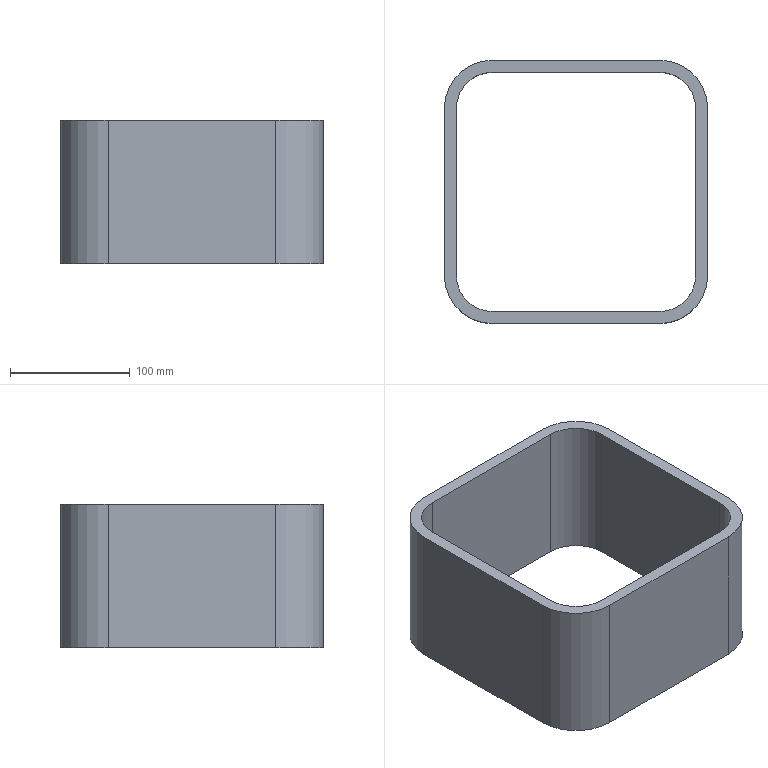Part | SolidWorks | features Extrusion 1 | 1 solid | 18 faces | box 220 x 220 x 120 mm | volume 935894 mm3 | plane 10 | cylinder 8 | commonest cylinder face diameters 60 x4 80 x4
STEP:
#1=CARTESIAN_POINT('',(-70.,110.,120.));
#2=VERTEX_POINT('',#1);
#3=CARTESIAN_POINT('',(-110.,70.,120.));
#4=VERTEX_POINT('',#3);
#5=CARTESIAN_POINT('',(-70.,70.,120.));
#6=DIRECTION('',(0.,0.,1.));
#7=DIRECTION('',(-1.,0.,0.));
#8=AXIS2_PLACEMENT_3D('',#5,#6,#7);
#9=CIRCLE('',#8,40.);
#10=EDGE_CURVE('',#2,#4,#9,.T.);
#11=ORIENTED_EDGE('',*,*,#10,.T.);
#12=CARTESIAN_POINT('',(-110.,-70.,120.));
#13=VERTEX_POINT('',#12);
#14=CARTESIAN_POINT('',(-110.,70.,120.));
#15=DIRECTION('',(0.,-1.,0.));
#16=VECTOR('',#15,1000.);
#17=LINE('',#14,#16);
#18=EDGE_CURVE('',#4,#13,#17,.T.);
#19=ORIENTED_EDGE('',*,*,#18,.T.);
#20=CARTESIAN_POINT('',(-70.,-110.,120.));
#21=VERTEX_POINT('',#20);
#22=CARTESIAN_POINT('',(-70.,-70.,120.));
#23=DIRECTION('',(0.,0.,1.));
#24=DIRECTION('',(-1.,0.,0.));
#25=AXIS2_PLACEMENT_3D('',#22,#23,#24);
#26=CIRCLE('',#25,40.);
#27=EDGE_CURVE('',#13,#21,#26,.T.);
#28=ORIENTED_EDGE('',*,*,#27,.T.);
#29=CARTESIAN_POINT('',(70.,-110.,120.));
#30=VERTEX_POINT('',#29);
#31=CARTESIAN_POINT('',(-70.,-110.,120.));
#32=DIRECTION('',(1.,0.,0.));
#33=VECTOR('',#32,1000.);
#34=LINE('',#31,#33);
#35=EDGE_CURVE('',#21,#30,#34,.T.);
#36=ORIENTED_EDGE('',*,*,#35,.T.);
#37=CARTESIAN_POINT('',(110.,-70.,120.));
#38=VERTEX_POINT('',#37);
#39=CARTESIAN_POINT('',(70.,-70.,120.));
#40=DIRECTION('',(0.,0.,1.));
#41=DIRECTION('',(1.,0.,0.));
#42=AXIS2_PLACEMENT_3D('',#39,#40,#41);
#43=CIRCLE('',#42,40.);
#44=EDGE_CURVE('',#30,#38,#43,.T.);
#45=ORIENTED_EDGE('',*,*,#44,.T.);
#46=CARTESIAN_POINT('',(110.,70.,120.));
#47=VERTEX_POINT('',#46);
#48=CARTESIAN_POINT('',(110.,70.,120.));
#49=DIRECTION('',(0.,1.,0.));
#50=VECTOR('',#49,1000.);
#51=LINE('',#48,#50);
#52=EDGE_CURVE('',#38,#47,#51,.T.);
#53=ORIENTED_EDGE('',*,*,#52,.T.);
#54=CARTESIAN_POINT('',(70.,110.,120.));
#55=VERTEX_POINT('',#54);
#56=CARTESIAN_POINT('',(70.,70.,120.));
#57=DIRECTION('',(0.,0.,1.));
#58=DIRECTION('',(1.,0.,0.));
#59=AXIS2_PLACEMENT_3D('',#56,#57,#58);
#60=CIRCLE('',#59,40.);
#61=EDGE_CURVE('',#47,#55,#60,.T.);
#62=ORIENTED_EDGE('',*,*,#61,.T.);
#63=CARTESIAN_POINT('',(-70.,110.,120.));
#64=DIRECTION('',(-1.,0.,0.));
#65=VECTOR('',#64,1000.);
#66=LINE('',#63,#65);
#67=EDGE_CURVE('',#55,#2,#66,.T.);
#68=ORIENTED_EDGE('',*,*,#67,.T.);
#69=EDGE_LOOP('',(#11,#19,#28,#36,#45,#53,#62,#68));
#70=FACE_OUTER_BOUND('',#69,.T.);
#71=CARTESIAN_POINT('',(70.,-100.,120.));
#72=VERTEX_POINT('',#71);
#73=CARTESIAN_POINT('',(100.,-70.,120.));
#74=VERTEX_POINT('',#73);
#75=CARTESIAN_POINT('',(70.,-70.,120.));
#76=DIRECTION('',(0.,0.,1.));
#77=DIRECTION('',(1.,0.,0.));
#78=AXIS2_PLACEMENT_3D('',#75,#76,#77);
#79=CIRCLE('',#78,30.);
#80=EDGE_CURVE('',#72,#74,#79,.T.);
#81=ORIENTED_EDGE('',*,*,#80,.F.);
#82=CARTESIAN_POINT('',(-70.,-100.,120.));
#83=VERTEX_POINT('',#82);
#84=CARTESIAN_POINT('',(-70.,-100.,120.));
#85=DIRECTION('',(1.,0.,0.));
#86=VECTOR('',#85,1000.);
#87=LINE('',#84,#86);
#88=EDGE_CURVE('',#83,#72,#87,.T.);
#89=ORIENTED_EDGE('',*,*,#88,.F.);
#90=CARTESIAN_POINT('',(-100.,-70.,120.));
#91=VERTEX_POINT('',#90);
#92=CARTESIAN_POINT('',(-70.,-70.,120.));
#93=DIRECTION('',(0.,0.,1.));
#94=DIRECTION('',(-1.,0.,0.));
#95=AXIS2_PLACEMENT_3D('',#92,#93,#94);
#96=CIRCLE('',#95,30.);
#97=EDGE_CURVE('',#91,#83,#96,.T.);
#98=ORIENTED_EDGE('',*,*,#97,.F.);
#99=CARTESIAN_POINT('',(-100.,70.,120.));
#100=VERTEX_POINT('',#99);
#101=CARTESIAN_POINT('',(-100.,70.,120.));
#102=DIRECTION('',(0.,-1.,0.));
#103=VECTOR('',#102,1000.);
#104=LINE('',#101,#103);
#105=EDGE_CURVE('',#100,#91,#104,.T.);
#106=ORIENTED_EDGE('',*,*,#105,.F.);
#107=CARTESIAN_POINT('',(-70.,100.,120.));
#108=VERTEX_POINT('',#107);
#109=CARTESIAN_POINT('',(-70.,70.,120.));
#110=DIRECTION('',(0.,0.,1.));
#111=DIRECTION('',(-1.,0.,0.));
#112=AXIS2_PLACEMENT_3D('',#109,#110,#111);
#113=CIRCLE('',#112,30.);
#114=EDGE_CURVE('',#108,#100,#113,.T.);
#115=ORIENTED_EDGE('',*,*,#114,.F.);
#116=CARTESIAN_POINT('',(70.,100.,120.));
#117=VERTEX_POINT('',#116);
#118=CARTESIAN_POINT('',(-70.,100.,120.));
#119=DIRECTION('',(-1.,0.,0.));
#120=VECTOR('',#119,1000.);
#121=LINE('',#118,#120);
#122=EDGE_CURVE('',#117,#108,#121,.T.);
#123=ORIENTED_EDGE('',*,*,#122,.F.);
#124=CARTESIAN_POINT('',(100.,70.,120.));
#125=VERTEX_POINT('',#124);
#126=CARTESIAN_POINT('',(70.,70.,120.));
#127=DIRECTION('',(0.,0.,1.));
#128=DIRECTION('',(1.,0.,0.));
#129=AXIS2_PLACEMENT_3D('',#126,#127,#128);
#130=CIRCLE('',#129,30.);
#131=EDGE_CURVE('',#125,#117,#130,.T.);
#132=ORIENTED_EDGE('',*,*,#131,.F.);
#133=CARTESIAN_POINT('',(100.,70.,120.));
#134=DIRECTION('',(0.,1.,0.));
#135=VECTOR('',#134,1000.);
#136=LINE('',#133,#135);
#137=EDGE_CURVE('',#74,#125,#136,.T.);
#138=ORIENTED_EDGE('',*,*,#137,.F.);
#139=EDGE_LOOP('',(#81,#89,#98,#106,#115,#123,#132,#138));
#140=FACE_BOUND('',#139,.T.);
#141=CARTESIAN_POINT('',(-70.,70.,120.));
#142=DIRECTION('',(0.,0.,-1.));
#143=DIRECTION('',(-1.,0.,0.));
#144=AXIS2_PLACEMENT_3D('',#141,#142,#143);
#145=PLANE('',#144);
#146=ADVANCED_FACE('',(#70,#140),#145,.F.);
#147=CARTESIAN_POINT('',(-70.,110.,0.));
#148=VERTEX_POINT('',#147);
#149=CARTESIAN_POINT('',(-110.,70.,0.));
#150=VERTEX_POINT('',#149);
#151=CARTESIAN_POINT('',(-70.,70.,0.));
#152=DIRECTION('',(0.,0.,1.));
#153=DIRECTION('',(-1.,0.,0.));
#154=AXIS2_PLACEMENT_3D('',#151,#152,#153);
#155=CIRCLE('',#154,40.);
#156=EDGE_CURVE('',#148,#150,#155,.T.);
#157=ORIENTED_EDGE('',*,*,#156,.F.);
#158=CARTESIAN_POINT('',(70.,110.,0.));
#159=VERTEX_POINT('',#158);
#160=CARTESIAN_POINT('',(-70.,110.,0.));
#161=DIRECTION('',(-1.,0.,0.));
#162=VECTOR('',#161,1000.);
#163=LINE('',#160,#162);
#164=EDGE_CURVE('',#159,#148,#163,.T.);
#165=ORIENTED_EDGE('',*,*,#164,.F.);
#166=CARTESIAN_POINT('',(110.,70.,0.));
#167=VERTEX_POINT('',#166);
#168=CARTESIAN_POINT('',(70.,70.,0.));
#169=DIRECTION('',(0.,0.,1.));
#170=DIRECTION('',(1.,0.,0.));
#171=AXIS2_PLACEMENT_3D('',#168,#169,#170);
#172=CIRCLE('',#171,40.);
#173=EDGE_CURVE('',#167,#159,#172,.T.);
#174=ORIENTED_EDGE('',*,*,#173,.F.);
#175=CARTESIAN_POINT('',(110.,-70.,0.));
#176=VERTEX_POINT('',#175);
#177=CARTESIAN_POINT('',(110.,70.,0.));
#178=DIRECTION('',(0.,1.,0.));
#179=VECTOR('',#178,1000.);
#180=LINE('',#177,#179);
#181=EDGE_CURVE('',#176,#167,#180,.T.);
#182=ORIENTED_EDGE('',*,*,#181,.F.);
#183=CARTESIAN_POINT('',(70.,-110.,0.));
#184=VERTEX_POINT('',#183);
#185=CARTESIAN_POINT('',(70.,-70.,0.));
#186=DIRECTION('',(0.,0.,1.));
#187=DIRECTION('',(1.,0.,0.));
#188=AXIS2_PLACEMENT_3D('',#185,#186,#187);
#189=CIRCLE('',#188,40.);
#190=EDGE_CURVE('',#184,#176,#189,.T.);
#191=ORIENTED_EDGE('',*,*,#190,.F.);
#192=CARTESIAN_POINT('',(-70.,-110.,0.));
#193=VERTEX_POINT('',#192);
#194=CARTESIAN_POINT('',(-70.,-110.,0.));
#195=DIRECTION('',(1.,0.,0.));
#196=VECTOR('',#195,1000.);
#197=LINE('',#194,#196);
#198=EDGE_CURVE('',#193,#184,#197,.T.);
#199=ORIENTED_EDGE('',*,*,#198,.F.);
#200=CARTESIAN_POINT('',(-110.,-70.,0.));
#201=VERTEX_POINT('',#200);
#202=CARTESIAN_POINT('',(-70.,-70.,0.));
#203=DIRECTION('',(0.,0.,1.));
#204=DIRECTION('',(-1.,0.,0.));
#205=AXIS2_PLACEMENT_3D('',#202,#203,#204);
#206=CIRCLE('',#205,40.);
#207=EDGE_CURVE('',#201,#193,#206,.T.);
#208=ORIENTED_EDGE('',*,*,#207,.F.);
#209=CARTESIAN_POINT('',(-110.,70.,0.));
#210=DIRECTION('',(0.,-1.,0.));
#211=VECTOR('',#210,1000.);
#212=LINE('',#209,#211);
#213=EDGE_CURVE('',#150,#201,#212,.T.);
#214=ORIENTED_EDGE('',*,*,#213,.F.);
#215=EDGE_LOOP('',(#157,#165,#174,#182,#191,#199,#208,#214));
#216=FACE_OUTER_BOUND('',#215,.T.);
#217=CARTESIAN_POINT('',(-70.,-100.,0.));
#218=VERTEX_POINT('',#217);
#219=CARTESIAN_POINT('',(70.,-100.,0.));
#220=VERTEX_POINT('',#219);
#221=CARTESIAN_POINT('',(-70.,-100.,0.));
#222=DIRECTION('',(1.,0.,0.));
#223=VECTOR('',#222,1000.);
#224=LINE('',#221,#223);
#225=EDGE_CURVE('',#218,#220,#224,.T.);
#226=ORIENTED_EDGE('',*,*,#225,.T.);
#227=CARTESIAN_POINT('',(100.,-70.,0.));
#228=VERTEX_POINT('',#227);
#229=CARTESIAN_POINT('',(70.,-70.,0.));
#230=DIRECTION('',(0.,0.,1.));
#231=DIRECTION('',(1.,0.,0.));
#232=AXIS2_PLACEMENT_3D('',#229,#230,#231);
#233=CIRCLE('',#232,30.);
#234=EDGE_CURVE('',#220,#228,#233,.T.);
#235=ORIENTED_EDGE('',*,*,#234,.T.);
#236=CARTESIAN_POINT('',(100.,70.,0.));
#237=VERTEX_POINT('',#236);
#238=CARTESIAN_POINT('',(100.,70.,0.));
#239=DIRECTION('',(0.,1.,0.));
#240=VECTOR('',#239,1000.);
#241=LINE('',#238,#240);
#242=EDGE_CURVE('',#228,#237,#241,.T.);
#243=ORIENTED_EDGE('',*,*,#242,.T.);
#244=CARTESIAN_POINT('',(70.,100.,0.));
#245=VERTEX_POINT('',#244);
#246=CARTESIAN_POINT('',(70.,70.,0.));
#247=DIRECTION('',(0.,0.,1.));
#248=DIRECTION('',(1.,0.,0.));
#249=AXIS2_PLACEMENT_3D('',#246,#247,#248);
#250=CIRCLE('',#249,30.);
#251=EDGE_CURVE('',#237,#245,#250,.T.);
#252=ORIENTED_EDGE('',*,*,#251,.T.);
#253=CARTESIAN_POINT('',(-70.,100.,0.));
#254=VERTEX_POINT('',#253);
#255=CARTESIAN_POINT('',(-70.,100.,0.));
#256=DIRECTION('',(-1.,0.,0.));
#257=VECTOR('',#256,1000.);
#258=LINE('',#255,#257);
#259=EDGE_CURVE('',#245,#254,#258,.T.);
#260=ORIENTED_EDGE('',*,*,#259,.T.);
#261=CARTESIAN_POINT('',(-100.,70.,0.));
#262=VERTEX_POINT('',#261);
#263=CARTESIAN_POINT('',(-70.,70.,0.));
#264=DIRECTION('',(0.,0.,1.));
#265=DIRECTION('',(-1.,0.,0.));
#266=AXIS2_PLACEMENT_3D('',#263,#264,#265);
#267=CIRCLE('',#266,30.);
#268=EDGE_CURVE('',#254,#262,#267,.T.);
#269=ORIENTED_EDGE('',*,*,#268,.T.);
#270=CARTESIAN_POINT('',(-100.,-70.,0.));
#271=VERTEX_POINT('',#270);
#272=CARTESIAN_POINT('',(-100.,70.,0.));
#273=DIRECTION('',(0.,-1.,0.));
#274=VECTOR('',#273,1000.);
#275=LINE('',#272,#274);
#276=EDGE_CURVE('',#262,#271,#275,.T.);
#277=ORIENTED_EDGE('',*,*,#276,.T.);
#278=CARTESIAN_POINT('',(-70.,-70.,0.));
#279=DIRECTION('',(0.,0.,1.));
#280=DIRECTION('',(-1.,0.,0.));
#281=AXIS2_PLACEMENT_3D('',#278,#279,#280);
#282=CIRCLE('',#281,30.);
#283=EDGE_CURVE('',#271,#218,#282,.T.);
#284=ORIENTED_EDGE('',*,*,#283,.T.);
#285=EDGE_LOOP('',(#226,#235,#243,#252,#260,#269,#277,#284));
#286=FACE_BOUND('',#285,.T.);
#287=CARTESIAN_POINT('',(-70.,70.,0.));
#288=DIRECTION('',(0.,0.,-1.));
#289=DIRECTION('',(-1.,0.,0.));
#290=AXIS2_PLACEMENT_3D('',#287,#288,#289);
#291=PLANE('',#290);
#292=ADVANCED_FACE('',(#216,#286),#291,.T.);
#293=ORIENTED_EDGE('',*,*,#156,.T.);
#294=CARTESIAN_POINT('',(-110.,70.,120.));
#295=DIRECTION('',(0.,0.,-1.));
#296=VECTOR('',#295,1000.);
#297=LINE('',#294,#296);
#298=EDGE_CURVE('',#4,#150,#297,.T.);
#299=ORIENTED_EDGE('',*,*,#298,.F.);
#300=ORIENTED_EDGE('',*,*,#10,.F.);
#301=CARTESIAN_POINT('',(-70.,110.,120.));
#302=DIRECTION('',(0.,0.,-1.));
#303=VECTOR('',#302,1000.);
#304=LINE('',#301,#303);
#305=EDGE_CURVE('',#2,#148,#304,.T.);
#306=ORIENTED_EDGE('',*,*,#305,.T.);
#307=EDGE_LOOP('',(#293,#299,#300,#306));
#308=FACE_OUTER_BOUND('',#307,.T.);
#309=CARTESIAN_POINT('',(-70.,70.,120.));
#310=DIRECTION('',(0.,0.,-1.));
#311=DIRECTION('',(-1.,0.,0.));
#312=AXIS2_PLACEMENT_3D('',#309,#310,#311);
#313=CYLINDRICAL_SURFACE('',#312,40.);
#314=ADVANCED_FACE('',(#308),#313,.T.);
#315=ORIENTED_EDGE('',*,*,#213,.T.);
#316=CARTESIAN_POINT('',(-110.,-70.,120.));
#317=DIRECTION('',(0.,0.,-1.));
#318=VECTOR('',#317,1000.);
#319=LINE('',#316,#318);
#320=EDGE_CURVE('',#13,#201,#319,.T.);
#321=ORIENTED_EDGE('',*,*,#320,.F.);
#322=ORIENTED_EDGE('',*,*,#18,.F.);
#323=ORIENTED_EDGE('',*,*,#298,.T.);
#324=EDGE_LOOP('',(#315,#321,#322,#323));
#325=FACE_OUTER_BOUND('',#324,.T.);
#326=CARTESIAN_POINT('',(-110.,70.,120.));
#327=DIRECTION('',(1.,0.,0.));
#328=DIRECTION('',(0.,1.,0.));
#329=AXIS2_PLACEMENT_3D('',#326,#327,#328);
#330=PLANE('',#329);
#331=ADVANCED_FACE('',(#325),#330,.F.);
#332=ORIENTED_EDGE('',*,*,#207,.T.);
#333=CARTESIAN_POINT('',(-70.,-110.,120.));
#334=DIRECTION('',(0.,0.,-1.));
#335=VECTOR('',#334,1000.);
#336=LINE('',#333,#335);
#337=EDGE_CURVE('',#21,#193,#336,.T.);
#338=ORIENTED_EDGE('',*,*,#337,.F.);
#339=ORIENTED_EDGE('',*,*,#27,.F.);
#340=ORIENTED_EDGE('',*,*,#320,.T.);
#341=EDGE_LOOP('',(#332,#338,#339,#340));
#342=FACE_OUTER_BOUND('',#341,.T.);
#343=CARTESIAN_POINT('',(-70.,-70.,120.));
#344=DIRECTION('',(0.,0.,-1.));
#345=DIRECTION('',(-1.,0.,0.));
#346=AXIS2_PLACEMENT_3D('',#343,#344,#345);
#347=CYLINDRICAL_SURFACE('',#346,40.);
#348=ADVANCED_FACE('',(#342),#347,.T.);
#349=ORIENTED_EDGE('',*,*,#198,.T.);
#350=CARTESIAN_POINT('',(70.,-110.,120.));
#351=DIRECTION('',(0.,0.,-1.));
#352=VECTOR('',#351,1000.);
#353=LINE('',#350,#352);
#354=EDGE_CURVE('',#30,#184,#353,.T.);
#355=ORIENTED_EDGE('',*,*,#354,.F.);
#356=ORIENTED_EDGE('',*,*,#35,.F.);
#357=ORIENTED_EDGE('',*,*,#337,.T.);
#358=EDGE_LOOP('',(#349,#355,#356,#357));
#359=FACE_OUTER_BOUND('',#358,.T.);
#360=CARTESIAN_POINT('',(-70.,-110.,120.));
#361=DIRECTION('',(0.,1.,0.));
#362=DIRECTION('',(-1.,0.,0.));
#363=AXIS2_PLACEMENT_3D('',#360,#361,#362);
#364=PLANE('',#363);
#365=ADVANCED_FACE('',(#359),#364,.F.);
#366=ORIENTED_EDGE('',*,*,#190,.T.);
#367=CARTESIAN_POINT('',(110.,-70.,120.));
#368=DIRECTION('',(0.,0.,-1.));
#369=VECTOR('',#368,1000.);
#370=LINE('',#367,#369);
#371=EDGE_CURVE('',#38,#176,#370,.T.);
#372=ORIENTED_EDGE('',*,*,#371,.F.);
#373=ORIENTED_EDGE('',*,*,#44,.F.);
#374=ORIENTED_EDGE('',*,*,#354,.T.);
#375=EDGE_LOOP('',(#366,#372,#373,#374));
#376=FACE_OUTER_BOUND('',#375,.T.);
#377=CARTESIAN_POINT('',(70.,-70.,120.));
#378=DIRECTION('',(0.,0.,-1.));
#379=DIRECTION('',(-1.,0.,0.));
#380=AXIS2_PLACEMENT_3D('',#377,#378,#379);
#381=CYLINDRICAL_SURFACE('',#380,40.);
#382=ADVANCED_FACE('',(#376),#381,.T.);
#383=ORIENTED_EDGE('',*,*,#181,.T.);
#384=CARTESIAN_POINT('',(110.,70.,120.));
#385=DIRECTION('',(0.,0.,-1.));
#386=VECTOR('',#385,1000.);
#387=LINE('',#384,#386);
#388=EDGE_CURVE('',#47,#167,#387,.T.);
#389=ORIENTED_EDGE('',*,*,#388,.F.);
#390=ORIENTED_EDGE('',*,*,#52,.F.);
#391=ORIENTED_EDGE('',*,*,#371,.T.);
#392=EDGE_LOOP('',(#383,#389,#390,#391));
#393=FACE_OUTER_BOUND('',#392,.T.);
#394=CARTESIAN_POINT('',(110.,70.,120.));
#395=DIRECTION('',(-1.,0.,0.));
#396=DIRECTION('',(0.,0.,1.));
#397=AXIS2_PLACEMENT_3D('',#394,#395,#396);
#398=PLANE('',#397);
#399=ADVANCED_FACE('',(#393),#398,.F.);
#400=ORIENTED_EDGE('',*,*,#173,.T.);
#401=CARTESIAN_POINT('',(70.,110.,120.));
#402=DIRECTION('',(0.,0.,-1.));
#403=VECTOR('',#402,1000.);
#404=LINE('',#401,#403);
#405=EDGE_CURVE('',#55,#159,#404,.T.);
#406=ORIENTED_EDGE('',*,*,#405,.F.);
#407=ORIENTED_EDGE('',*,*,#61,.F.);
#408=ORIENTED_EDGE('',*,*,#388,.T.);
#409=EDGE_LOOP('',(#400,#406,#407,#408));
#410=FACE_OUTER_BOUND('',#409,.T.);
#411=CARTESIAN_POINT('',(70.,70.,120.));
#412=DIRECTION('',(0.,0.,-1.));
#413=DIRECTION('',(-1.,0.,0.));
#414=AXIS2_PLACEMENT_3D('',#411,#412,#413);
#415=CYLINDRICAL_SURFACE('',#414,40.);
#416=ADVANCED_FACE('',(#410),#415,.T.);
#417=ORIENTED_EDGE('',*,*,#164,.T.);
#418=ORIENTED_EDGE('',*,*,#305,.F.);
#419=ORIENTED_EDGE('',*,*,#67,.F.);
#420=ORIENTED_EDGE('',*,*,#405,.T.);
#421=EDGE_LOOP('',(#417,#418,#419,#420));
#422=FACE_OUTER_BOUND('',#421,.T.);
#423=CARTESIAN_POINT('',(-70.,110.,120.));
#424=DIRECTION('',(0.,-1.,0.));
#425=DIRECTION('',(0.,0.,-1.));
#426=AXIS2_PLACEMENT_3D('',#423,#424,#425);
#427=PLANE('',#426);
#428=ADVANCED_FACE('',(#422),#427,.F.);
#429=ORIENTED_EDGE('',*,*,#234,.F.);
#430=CARTESIAN_POINT('',(70.,-100.,120.));
#431=DIRECTION('',(0.,0.,-1.));
#432=VECTOR('',#431,1000.);
#433=LINE('',#430,#432);
#434=EDGE_CURVE('',#72,#220,#433,.T.);
#435=ORIENTED_EDGE('',*,*,#434,.F.);
#436=ORIENTED_EDGE('',*,*,#80,.T.);
#437=CARTESIAN_POINT('',(100.,-70.,120.));
#438=DIRECTION('',(0.,0.,-1.));
#439=VECTOR('',#438,1000.);
#440=LINE('',#437,#439);
#441=EDGE_CURVE('',#74,#228,#440,.T.);
#442=ORIENTED_EDGE('',*,*,#441,.T.);
#443=EDGE_LOOP('',(#429,#435,#436,#442));
#444=FACE_OUTER_BOUND('',#443,.T.);
#445=CARTESIAN_POINT('',(70.,-70.,120.));
#446=DIRECTION('',(0.,0.,-1.));
#447=DIRECTION('',(-1.,0.,0.));
#448=AXIS2_PLACEMENT_3D('',#445,#446,#447);
#449=CYLINDRICAL_SURFACE('',#448,30.);
#450=ADVANCED_FACE('',(#444),#449,.F.);
#451=ORIENTED_EDGE('',*,*,#242,.F.);
#452=ORIENTED_EDGE('',*,*,#441,.F.);
#453=ORIENTED_EDGE('',*,*,#137,.T.);
#454=CARTESIAN_POINT('',(100.,70.,120.));
#455=DIRECTION('',(0.,0.,-1.));
#456=VECTOR('',#455,1000.);
#457=LINE('',#454,#456);
#458=EDGE_CURVE('',#125,#237,#457,.T.);
#459=ORIENTED_EDGE('',*,*,#458,.T.);
#460=EDGE_LOOP('',(#451,#452,#453,#459));
#461=FACE_OUTER_BOUND('',#460,.T.);
#462=CARTESIAN_POINT('',(100.,70.,120.));
#463=DIRECTION('',(-1.,0.,0.));
#464=DIRECTION('',(0.,-1.,0.));
#465=AXIS2_PLACEMENT_3D('',#462,#463,#464);
#466=PLANE('',#465);
#467=ADVANCED_FACE('',(#461),#466,.T.);
#468=ORIENTED_EDGE('',*,*,#251,.F.);
#469=ORIENTED_EDGE('',*,*,#458,.F.);
#470=ORIENTED_EDGE('',*,*,#131,.T.);
#471=CARTESIAN_POINT('',(70.,100.,120.));
#472=DIRECTION('',(0.,0.,-1.));
#473=VECTOR('',#472,1000.);
#474=LINE('',#471,#473);
#475=EDGE_CURVE('',#117,#245,#474,.T.);
#476=ORIENTED_EDGE('',*,*,#475,.T.);
#477=EDGE_LOOP('',(#468,#469,#470,#476));
#478=FACE_OUTER_BOUND('',#477,.T.);
#479=CARTESIAN_POINT('',(70.,70.,120.));
#480=DIRECTION('',(0.,0.,-1.));
#481=DIRECTION('',(-1.,0.,0.));
#482=AXIS2_PLACEMENT_3D('',#479,#480,#481);
#483=CYLINDRICAL_SURFACE('',#482,30.);
#484=ADVANCED_FACE('',(#478),#483,.F.);
#485=ORIENTED_EDGE('',*,*,#259,.F.);
#486=ORIENTED_EDGE('',*,*,#475,.F.);
#487=ORIENTED_EDGE('',*,*,#122,.T.);
#488=CARTESIAN_POINT('',(-70.,100.,120.));
#489=DIRECTION('',(0.,0.,-1.));
#490=VECTOR('',#489,1000.);
#491=LINE('',#488,#490);
#492=EDGE_CURVE('',#108,#254,#491,.T.);
#493=ORIENTED_EDGE('',*,*,#492,.T.);
#494=EDGE_LOOP('',(#485,#486,#487,#493));
#495=FACE_OUTER_BOUND('',#494,.T.);
#496=CARTESIAN_POINT('',(-70.,100.,120.));
#497=DIRECTION('',(0.,-1.,0.));
#498=DIRECTION('',(0.,0.,-1.));
#499=AXIS2_PLACEMENT_3D('',#496,#497,#498);
#500=PLANE('',#499);
#501=ADVANCED_FACE('',(#495),#500,.T.);
#502=ORIENTED_EDGE('',*,*,#268,.F.);
#503=ORIENTED_EDGE('',*,*,#492,.F.);
#504=ORIENTED_EDGE('',*,*,#114,.T.);
#505=CARTESIAN_POINT('',(-100.,70.,120.));
#506=DIRECTION('',(0.,0.,-1.));
#507=VECTOR('',#506,1000.);
#508=LINE('',#505,#507);
#509=EDGE_CURVE('',#100,#262,#508,.T.);
#510=ORIENTED_EDGE('',*,*,#509,.T.);
#511=EDGE_LOOP('',(#502,#503,#504,#510));
#512=FACE_OUTER_BOUND('',#511,.T.);
#513=CARTESIAN_POINT('',(-70.,70.,120.));
#514=DIRECTION('',(0.,0.,-1.));
#515=DIRECTION('',(-1.,0.,0.));
#516=AXIS2_PLACEMENT_3D('',#513,#514,#515);
#517=CYLINDRICAL_SURFACE('',#516,30.);
#518=ADVANCED_FACE('',(#512),#517,.F.);
#519=ORIENTED_EDGE('',*,*,#276,.F.);
#520=ORIENTED_EDGE('',*,*,#509,.F.);
#521=ORIENTED_EDGE('',*,*,#105,.T.);
#522=CARTESIAN_POINT('',(-100.,-70.,120.));
#523=DIRECTION('',(0.,0.,-1.));
#524=VECTOR('',#523,1000.);
#525=LINE('',#522,#524);
#526=EDGE_CURVE('',#91,#271,#525,.T.);
#527=ORIENTED_EDGE('',*,*,#526,.T.);
#528=EDGE_LOOP('',(#519,#520,#521,#527));
#529=FACE_OUTER_BOUND('',#528,.T.);
#530=CARTESIAN_POINT('',(-100.,70.,120.));
#531=DIRECTION('',(1.,0.,0.));
#532=DIRECTION('',(0.,0.,-1.));
#533=AXIS2_PLACEMENT_3D('',#530,#531,#532);
#534=PLANE('',#533);
#535=ADVANCED_FACE('',(#529),#534,.T.);
#536=ORIENTED_EDGE('',*,*,#283,.F.);
#537=ORIENTED_EDGE('',*,*,#526,.F.);
#538=ORIENTED_EDGE('',*,*,#97,.T.);
#539=CARTESIAN_POINT('',(-70.,-100.,120.));
#540=DIRECTION('',(0.,0.,-1.));
#541=VECTOR('',#540,1000.);
#542=LINE('',#539,#541);
#543=EDGE_CURVE('',#83,#218,#542,.T.);
#544=ORIENTED_EDGE('',*,*,#543,.T.);
#545=EDGE_LOOP('',(#536,#537,#538,#544));
#546=FACE_OUTER_BOUND('',#545,.T.);
#547=CARTESIAN_POINT('',(-70.,-70.,120.));
#548=DIRECTION('',(0.,0.,-1.));
#549=DIRECTION('',(-1.,0.,0.));
#550=AXIS2_PLACEMENT_3D('',#547,#548,#549);
#551=CYLINDRICAL_SURFACE('',#550,30.);
#552=ADVANCED_FACE('',(#546),#551,.F.);
#553=ORIENTED_EDGE('',*,*,#225,.F.);
#554=ORIENTED_EDGE('',*,*,#543,.F.);
#555=ORIENTED_EDGE('',*,*,#88,.T.);
#556=ORIENTED_EDGE('',*,*,#434,.T.);
#557=EDGE_LOOP('',(#553,#554,#555,#556));
#558=FACE_OUTER_BOUND('',#557,.T.);
#559=CARTESIAN_POINT('',(-70.,-100.,120.));
#560=DIRECTION('',(0.,1.,0.));
#561=DIRECTION('',(0.,0.,1.));
#562=AXIS2_PLACEMENT_3D('',#559,#560,#561);
#563=PLANE('',#562);
#564=ADVANCED_FACE('',(#558),#563,.T.);
#565=CLOSED_SHELL('',(#146,#292,#314,#331,#348,#365,#382,#399,#416,#428,#450,#467,#484,#501,#518,#535,#552,#564));
#566=MANIFOLD_SOLID_BREP('',#565);
#567=CARTESIAN_POINT('',(0.,0.,0.));
#568=DIRECTION('',(0.,0.,1.));
#569=DIRECTION('',(1.,0.,0.));
#570=AXIS2_PLACEMENT_3D('',#567,#568,#569);
#571=(LENGTH_UNIT()NAMED_UNIT(*)SI_UNIT(.MILLI.,.METRE.));
#572=UNCERTAINTY_MEASURE_WITH_UNIT(LENGTH_MEASURE(0.00001),#571,'','');
#573=(NAMED_UNIT(*)PLANE_ANGLE_UNIT()SI_UNIT($,.RADIAN.));
#574=(NAMED_UNIT(*)SI_UNIT($,.STERADIAN.)SOLID_ANGLE_UNIT());
#575=(GEOMETRIC_REPRESENTATION_CONTEXT(3)GLOBAL_UNCERTAINTY_ASSIGNED_CONTEXT((#572))GLOBAL_UNIT_ASSIGNED_CONTEXT((#571,#573,#574))REPRESENTATION_CONTEXT('',''));
#576=ADVANCED_BREP_SHAPE_REPRESENTATION('',(#566,#570),#575);